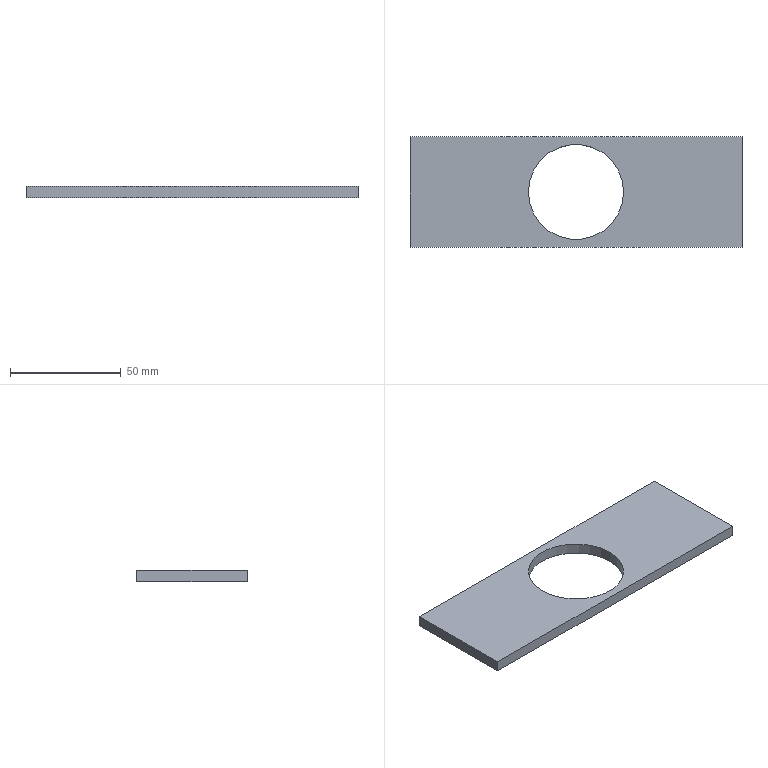Part | SolidWorks | features FlatPattern 1, ICE 1, SMBaseFlange 1, SheetMetal 1 | 1 solid | 8 faces | box 150 x 50 x 5 mm | volume 30239 mm3 | plane 6 | cylinder 2 | commonest cylinder face diameters 43 x2
STEP:
#1=CARTESIAN_POINT('',(-21.5,0.,0.));
#2=VERTEX_POINT('',#1);
#3=CARTESIAN_POINT('',(21.5,0.,0.));
#4=VERTEX_POINT('',#3);
#5=CARTESIAN_POINT('',(0.,0.,0.));
#6=DIRECTION('',(0.,0.,1.));
#7=DIRECTION('',(1.,0.,0.));
#8=AXIS2_PLACEMENT_3D('',#5,#6,#7);
#9=CIRCLE('',#8,21.5);
#10=EDGE_CURVE('',#2,#4,#9,.T.);
#11=ORIENTED_EDGE('',*,*,#10,.T.);
#12=CARTESIAN_POINT('',(21.5,0.,-5.));
#13=VERTEX_POINT('',#12);
#14=CARTESIAN_POINT('',(21.5,0.,5.));
#15=DIRECTION('',(0.,0.,-1.));
#16=VECTOR('',#15,1000.);
#17=LINE('',#14,#16);
#18=EDGE_CURVE('',#4,#13,#17,.T.);
#19=ORIENTED_EDGE('',*,*,#18,.T.);
#20=CARTESIAN_POINT('',(-21.5,0.,-5.));
#21=VERTEX_POINT('',#20);
#22=CARTESIAN_POINT('',(0.,0.,-5.));
#23=DIRECTION('',(0.,0.,-1.));
#24=DIRECTION('',(-1.,0.,0.));
#25=AXIS2_PLACEMENT_3D('',#22,#23,#24);
#26=CIRCLE('',#25,21.5);
#27=EDGE_CURVE('',#13,#21,#26,.T.);
#28=ORIENTED_EDGE('',*,*,#27,.T.);
#29=CARTESIAN_POINT('',(-21.5,0.,5.));
#30=DIRECTION('',(0.,0.,-1.));
#31=VECTOR('',#30,1000.);
#32=LINE('',#29,#31);
#33=EDGE_CURVE('',#2,#21,#32,.T.);
#34=ORIENTED_EDGE('',*,*,#33,.F.);
#35=EDGE_LOOP('',(#11,#19,#28,#34));
#36=FACE_OUTER_BOUND('',#35,.T.);
#37=CARTESIAN_POINT('',(0.,0.,5.));
#38=DIRECTION('',(0.,0.,-1.));
#39=DIRECTION('',(-1.,0.,0.));
#40=AXIS2_PLACEMENT_3D('',#37,#38,#39);
#41=CYLINDRICAL_SURFACE('',#40,21.5);
#42=ADVANCED_FACE('',(#36),#41,.F.);
#43=CARTESIAN_POINT('',(75.,-25.,0.));
#44=VERTEX_POINT('',#43);
#45=CARTESIAN_POINT('',(75.,25.,0.));
#46=VERTEX_POINT('',#45);
#47=CARTESIAN_POINT('',(75.,25.,0.));
#48=DIRECTION('',(0.,1.,0.));
#49=VECTOR('',#48,1000.);
#50=LINE('',#47,#49);
#51=EDGE_CURVE('',#44,#46,#50,.T.);
#52=ORIENTED_EDGE('',*,*,#51,.F.);
#53=CARTESIAN_POINT('',(75.,-25.,-5.));
#54=VERTEX_POINT('',#53);
#55=CARTESIAN_POINT('',(75.,-25.,-5.));
#56=DIRECTION('',(0.,0.,1.));
#57=VECTOR('',#56,1000.);
#58=LINE('',#55,#57);
#59=EDGE_CURVE('',#54,#44,#58,.T.);
#60=ORIENTED_EDGE('',*,*,#59,.F.);
#61=CARTESIAN_POINT('',(75.,25.,-5.));
#62=VERTEX_POINT('',#61);
#63=CARTESIAN_POINT('',(75.,25.,-5.));
#64=DIRECTION('',(0.,1.,0.));
#65=VECTOR('',#64,1000.);
#66=LINE('',#63,#65);
#67=EDGE_CURVE('',#54,#62,#66,.T.);
#68=ORIENTED_EDGE('',*,*,#67,.T.);
#69=CARTESIAN_POINT('',(75.,25.,-5.));
#70=DIRECTION('',(0.,0.,1.));
#71=VECTOR('',#70,1000.);
#72=LINE('',#69,#71);
#73=EDGE_CURVE('',#62,#46,#72,.T.);
#74=ORIENTED_EDGE('',*,*,#73,.T.);
#75=EDGE_LOOP('',(#52,#60,#68,#74));
#76=FACE_OUTER_BOUND('',#75,.T.);
#77=CARTESIAN_POINT('',(75.,25.,-5.));
#78=DIRECTION('',(1.,0.,0.));
#79=DIRECTION('',(0.,1.,0.));
#80=AXIS2_PLACEMENT_3D('',#77,#78,#79);
#81=PLANE('',#80);
#82=ADVANCED_FACE('',(#76),#81,.T.);
#83=CARTESIAN_POINT('',(-75.,-25.,0.));
#84=VERTEX_POINT('',#83);
#85=CARTESIAN_POINT('',(-75.,-25.,0.));
#86=DIRECTION('',(1.,0.,0.));
#87=VECTOR('',#86,1000.);
#88=LINE('',#85,#87);
#89=EDGE_CURVE('',#84,#44,#88,.T.);
#90=ORIENTED_EDGE('',*,*,#89,.F.);
#91=CARTESIAN_POINT('',(-75.,-25.,-5.));
#92=VERTEX_POINT('',#91);
#93=CARTESIAN_POINT('',(-75.,-25.,-5.));
#94=DIRECTION('',(0.,0.,1.));
#95=VECTOR('',#94,1000.);
#96=LINE('',#93,#95);
#97=EDGE_CURVE('',#92,#84,#96,.T.);
#98=ORIENTED_EDGE('',*,*,#97,.F.);
#99=CARTESIAN_POINT('',(-75.,-25.,-5.));
#100=DIRECTION('',(1.,0.,0.));
#101=VECTOR('',#100,1000.);
#102=LINE('',#99,#101);
#103=EDGE_CURVE('',#92,#54,#102,.T.);
#104=ORIENTED_EDGE('',*,*,#103,.T.);
#105=ORIENTED_EDGE('',*,*,#59,.T.);
#106=EDGE_LOOP('',(#90,#98,#104,#105));
#107=FACE_OUTER_BOUND('',#106,.T.);
#108=CARTESIAN_POINT('',(-75.,-25.,-5.));
#109=DIRECTION('',(0.,-1.,0.));
#110=DIRECTION('',(0.,0.,-1.));
#111=AXIS2_PLACEMENT_3D('',#108,#109,#110);
#112=PLANE('',#111);
#113=ADVANCED_FACE('',(#107),#112,.T.);
#114=CARTESIAN_POINT('',(-75.,25.,0.));
#115=VERTEX_POINT('',#114);
#116=CARTESIAN_POINT('',(-75.,25.,0.));
#117=DIRECTION('',(0.,-1.,0.));
#118=VECTOR('',#117,1000.);
#119=LINE('',#116,#118);
#120=EDGE_CURVE('',#115,#84,#119,.T.);
#121=ORIENTED_EDGE('',*,*,#120,.F.);
#122=CARTESIAN_POINT('',(-75.,25.,-5.));
#123=VERTEX_POINT('',#122);
#124=CARTESIAN_POINT('',(-75.,25.,-5.));
#125=DIRECTION('',(0.,0.,1.));
#126=VECTOR('',#125,1000.);
#127=LINE('',#124,#126);
#128=EDGE_CURVE('',#123,#115,#127,.T.);
#129=ORIENTED_EDGE('',*,*,#128,.F.);
#130=CARTESIAN_POINT('',(-75.,25.,-5.));
#131=DIRECTION('',(0.,-1.,0.));
#132=VECTOR('',#131,1000.);
#133=LINE('',#130,#132);
#134=EDGE_CURVE('',#123,#92,#133,.T.);
#135=ORIENTED_EDGE('',*,*,#134,.T.);
#136=ORIENTED_EDGE('',*,*,#97,.T.);
#137=EDGE_LOOP('',(#121,#129,#135,#136));
#138=FACE_OUTER_BOUND('',#137,.T.);
#139=CARTESIAN_POINT('',(-75.,25.,-5.));
#140=DIRECTION('',(-1.,0.,0.));
#141=DIRECTION('',(0.,0.,1.));
#142=AXIS2_PLACEMENT_3D('',#139,#140,#141);
#143=PLANE('',#142);
#144=ADVANCED_FACE('',(#138),#143,.T.);
#145=CARTESIAN_POINT('',(-75.,25.,0.));
#146=DIRECTION('',(-1.,0.,0.));
#147=VECTOR('',#146,1000.);
#148=LINE('',#145,#147);
#149=EDGE_CURVE('',#46,#115,#148,.T.);
#150=ORIENTED_EDGE('',*,*,#149,.F.);
#151=ORIENTED_EDGE('',*,*,#73,.F.);
#152=CARTESIAN_POINT('',(-75.,25.,-5.));
#153=DIRECTION('',(-1.,0.,0.));
#154=VECTOR('',#153,1000.);
#155=LINE('',#152,#154);
#156=EDGE_CURVE('',#62,#123,#155,.T.);
#157=ORIENTED_EDGE('',*,*,#156,.T.);
#158=ORIENTED_EDGE('',*,*,#128,.T.);
#159=EDGE_LOOP('',(#150,#151,#157,#158));
#160=FACE_OUTER_BOUND('',#159,.T.);
#161=CARTESIAN_POINT('',(-75.,25.,-5.));
#162=DIRECTION('',(0.,1.,0.));
#163=DIRECTION('',(0.,0.,1.));
#164=AXIS2_PLACEMENT_3D('',#161,#162,#163);
#165=PLANE('',#164);
#166=ADVANCED_FACE('',(#160),#165,.T.);
#167=CARTESIAN_POINT('',(0.,0.,-5.));
#168=DIRECTION('',(0.,0.,-1.));
#169=DIRECTION('',(-1.,0.,0.));
#170=AXIS2_PLACEMENT_3D('',#167,#168,#169);
#171=CIRCLE('',#170,21.5);
#172=EDGE_CURVE('',#21,#13,#171,.T.);
#173=ORIENTED_EDGE('',*,*,#172,.F.);
#174=ORIENTED_EDGE('',*,*,#27,.F.);
#175=EDGE_LOOP('',(#173,#174));
#176=FACE_BOUND('',#175,.T.);
#177=ORIENTED_EDGE('',*,*,#67,.F.);
#178=ORIENTED_EDGE('',*,*,#103,.F.);
#179=ORIENTED_EDGE('',*,*,#134,.F.);
#180=ORIENTED_EDGE('',*,*,#156,.F.);
#181=EDGE_LOOP('',(#177,#178,#179,#180));
#182=FACE_OUTER_BOUND('',#181,.T.);
#183=CARTESIAN_POINT('',(0.,0.,-5.));
#184=DIRECTION('',(0.,0.,1.));
#185=DIRECTION('',(1.,0.,0.));
#186=AXIS2_PLACEMENT_3D('',#183,#184,#185);
#187=PLANE('',#186);
#188=ADVANCED_FACE('',(#176,#182),#187,.F.);
#189=ORIENTED_EDGE('',*,*,#10,.F.);
#190=CARTESIAN_POINT('',(0.,0.,0.));
#191=DIRECTION('',(0.,0.,1.));
#192=DIRECTION('',(1.,0.,0.));
#193=AXIS2_PLACEMENT_3D('',#190,#191,#192);
#194=CIRCLE('',#193,21.5);
#195=EDGE_CURVE('',#4,#2,#194,.T.);
#196=ORIENTED_EDGE('',*,*,#195,.F.);
#197=EDGE_LOOP('',(#189,#196));
#198=FACE_BOUND('',#197,.T.);
#199=ORIENTED_EDGE('',*,*,#51,.T.);
#200=ORIENTED_EDGE('',*,*,#149,.T.);
#201=ORIENTED_EDGE('',*,*,#120,.T.);
#202=ORIENTED_EDGE('',*,*,#89,.T.);
#203=EDGE_LOOP('',(#199,#200,#201,#202));
#204=FACE_OUTER_BOUND('',#203,.T.);
#205=CARTESIAN_POINT('',(0.,0.,0.));
#206=DIRECTION('',(0.,0.,1.));
#207=DIRECTION('',(1.,0.,0.));
#208=AXIS2_PLACEMENT_3D('',#205,#206,#207);
#209=PLANE('',#208);
#210=ADVANCED_FACE('',(#198,#204),#209,.T.);
#211=ORIENTED_EDGE('',*,*,#18,.F.);
#212=ORIENTED_EDGE('',*,*,#195,.T.);
#213=ORIENTED_EDGE('',*,*,#33,.T.);
#214=ORIENTED_EDGE('',*,*,#172,.T.);
#215=EDGE_LOOP('',(#211,#212,#213,#214));
#216=FACE_OUTER_BOUND('',#215,.T.);
#217=CARTESIAN_POINT('',(0.,0.,5.));
#218=DIRECTION('',(0.,0.,-1.));
#219=DIRECTION('',(-1.,0.,0.));
#220=AXIS2_PLACEMENT_3D('',#217,#218,#219);
#221=CYLINDRICAL_SURFACE('',#220,21.5);
#222=ADVANCED_FACE('',(#216),#221,.F.);
#223=CLOSED_SHELL('',(#42,#82,#113,#144,#166,#188,#210,#222));
#224=MANIFOLD_SOLID_BREP('',#223);
#225=CARTESIAN_POINT('',(0.,0.,0.));
#226=DIRECTION('',(0.,0.,1.));
#227=DIRECTION('',(1.,0.,0.));
#228=AXIS2_PLACEMENT_3D('',#225,#226,#227);
#229=(LENGTH_UNIT()NAMED_UNIT(*)SI_UNIT(.MILLI.,.METRE.));
#230=UNCERTAINTY_MEASURE_WITH_UNIT(LENGTH_MEASURE(0.00001),#229,'','');
#231=(NAMED_UNIT(*)PLANE_ANGLE_UNIT()SI_UNIT($,.RADIAN.));
#232=(NAMED_UNIT(*)SI_UNIT($,.STERADIAN.)SOLID_ANGLE_UNIT());
#233=(GEOMETRIC_REPRESENTATION_CONTEXT(3)GLOBAL_UNCERTAINTY_ASSIGNED_CONTEXT((#230))GLOBAL_UNIT_ASSIGNED_CONTEXT((#229,#231,#232))REPRESENTATION_CONTEXT('',''));
#234=ADVANCED_BREP_SHAPE_REPRESENTATION('',(#224,#228),#233);